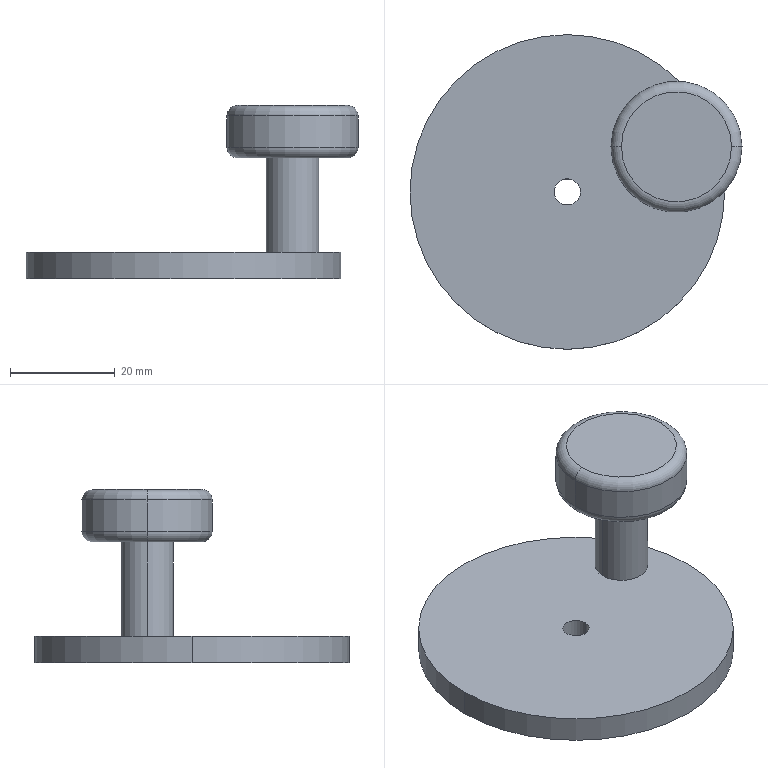Part | SolidWorks | features ICE 3, Extrusion 1, Fillet 1 | 1 solid | 16 faces | box 63.316 x 60 x 33 mm | volume 20231 mm3 | cylinder 8 | torus 4 | plane 4 | commonest cylinder face diameters 5 x2 10 x2 25 x2 60 x2
STEP:
#1=CARTESIAN_POINT('',(8.316,8.573,31.));
#2=VERTEX_POINT('',#1);
#3=CARTESIAN_POINT('',(33.316,8.573,31.));
#4=VERTEX_POINT('',#3);
#5=CARTESIAN_POINT('',(20.816,8.573,31.));
#6=DIRECTION('',(0.,0.,-1.));
#7=DIRECTION('',(1.,0.,0.));
#8=AXIS2_PLACEMENT_3D('',#5,#6,#7);
#9=CIRCLE('',#8,12.5);
#10=EDGE_CURVE('',#2,#4,#9,.T.);
#11=ORIENTED_EDGE('',*,*,#10,.F.);
#12=CARTESIAN_POINT('',(10.316,8.573,33.));
#13=VERTEX_POINT('',#12);
#14=CARTESIAN_POINT('',(10.316,8.573,31.));
#15=DIRECTION('',(0.,1.,0.));
#16=DIRECTION('',(-1.,0.,0.));
#17=AXIS2_PLACEMENT_3D('',#14,#15,#16);
#18=CIRCLE('',#17,2.);
#19=EDGE_CURVE('',#2,#13,#18,.T.);
#20=ORIENTED_EDGE('',*,*,#19,.T.);
#21=CARTESIAN_POINT('',(31.316,8.573,33.));
#22=VERTEX_POINT('',#21);
#23=CARTESIAN_POINT('',(20.816,8.573,33.));
#24=DIRECTION('',(0.,0.,1.));
#25=DIRECTION('',(1.,0.,0.));
#26=AXIS2_PLACEMENT_3D('',#23,#24,#25);
#27=CIRCLE('',#26,10.5);
#28=EDGE_CURVE('',#22,#13,#27,.T.);
#29=ORIENTED_EDGE('',*,*,#28,.F.);
#30=CARTESIAN_POINT('',(31.316,8.573,31.));
#31=DIRECTION('',(0.,-1.,0.));
#32=DIRECTION('',(0.,0.,-1.));
#33=AXIS2_PLACEMENT_3D('',#30,#31,#32);
#34=CIRCLE('',#33,2.);
#35=EDGE_CURVE('',#4,#22,#34,.T.);
#36=ORIENTED_EDGE('',*,*,#35,.F.);
#37=EDGE_LOOP('',(#11,#20,#29,#36));
#38=FACE_OUTER_BOUND('',#37,.T.);
#39=CARTESIAN_POINT('',(20.816,8.573,31.));
#40=DIRECTION('',(0.,0.,1.));
#41=DIRECTION('',(1.,0.,0.));
#42=AXIS2_PLACEMENT_3D('',#39,#40,#41);
#43=TOROIDAL_SURFACE('',#42,10.5,2.);
#44=ADVANCED_FACE('',(#38),#43,.T.);
#45=CARTESIAN_POINT('',(10.316,8.573,23.));
#46=VERTEX_POINT('',#45);
#47=CARTESIAN_POINT('',(31.316,8.573,23.));
#48=VERTEX_POINT('',#47);
#49=CARTESIAN_POINT('',(20.816,8.573,23.));
#50=DIRECTION('',(0.,0.,-1.));
#51=DIRECTION('',(1.,0.,0.));
#52=AXIS2_PLACEMENT_3D('',#49,#50,#51);
#53=CIRCLE('',#52,10.5);
#54=EDGE_CURVE('',#46,#48,#53,.T.);
#55=ORIENTED_EDGE('',*,*,#54,.F.);
#56=CARTESIAN_POINT('',(8.316,8.573,25.));
#57=VERTEX_POINT('',#56);
#58=CARTESIAN_POINT('',(10.316,8.573,25.));
#59=DIRECTION('',(0.,1.,0.));
#60=DIRECTION('',(-1.,0.,0.));
#61=AXIS2_PLACEMENT_3D('',#58,#59,#60);
#62=CIRCLE('',#61,2.);
#63=EDGE_CURVE('',#46,#57,#62,.T.);
#64=ORIENTED_EDGE('',*,*,#63,.T.);
#65=CARTESIAN_POINT('',(33.316,8.573,25.));
#66=VERTEX_POINT('',#65);
#67=CARTESIAN_POINT('',(20.816,8.573,25.));
#68=DIRECTION('',(0.,0.,1.));
#69=DIRECTION('',(1.,0.,0.));
#70=AXIS2_PLACEMENT_3D('',#67,#68,#69);
#71=CIRCLE('',#70,12.5);
#72=EDGE_CURVE('',#66,#57,#71,.T.);
#73=ORIENTED_EDGE('',*,*,#72,.F.);
#74=CARTESIAN_POINT('',(31.316,8.573,25.));
#75=DIRECTION('',(0.,-1.,0.));
#76=DIRECTION('',(0.,0.,-1.));
#77=AXIS2_PLACEMENT_3D('',#74,#75,#76);
#78=CIRCLE('',#77,2.);
#79=EDGE_CURVE('',#48,#66,#78,.T.);
#80=ORIENTED_EDGE('',*,*,#79,.F.);
#81=EDGE_LOOP('',(#55,#64,#73,#80));
#82=FACE_OUTER_BOUND('',#81,.T.);
#83=CARTESIAN_POINT('',(20.816,8.573,25.));
#84=DIRECTION('',(0.,0.,1.));
#85=DIRECTION('',(1.,0.,0.));
#86=AXIS2_PLACEMENT_3D('',#83,#84,#85);
#87=TOROIDAL_SURFACE('',#86,10.5,2.);
#88=ADVANCED_FACE('',(#82),#87,.T.);
#89=ORIENTED_EDGE('',*,*,#10,.T.);
#90=CARTESIAN_POINT('',(33.316,8.573,33.));
#91=DIRECTION('',(0.,0.,-1.));
#92=VECTOR('',#91,1000.);
#93=LINE('',#90,#92);
#94=EDGE_CURVE('',#4,#66,#93,.T.);
#95=ORIENTED_EDGE('',*,*,#94,.T.);
#96=ORIENTED_EDGE('',*,*,#72,.T.);
#97=CARTESIAN_POINT('',(8.316,8.573,33.));
#98=DIRECTION('',(0.,0.,-1.));
#99=VECTOR('',#98,1000.);
#100=LINE('',#97,#99);
#101=EDGE_CURVE('',#2,#57,#100,.T.);
#102=ORIENTED_EDGE('',*,*,#101,.F.);
#103=EDGE_LOOP('',(#89,#95,#96,#102));
#104=FACE_OUTER_BOUND('',#103,.T.);
#105=CARTESIAN_POINT('',(20.816,8.573,33.));
#106=DIRECTION('',(0.,0.,-1.));
#107=DIRECTION('',(-1.,0.,0.));
#108=AXIS2_PLACEMENT_3D('',#105,#106,#107);
#109=CYLINDRICAL_SURFACE('',#108,12.5);
#110=ADVANCED_FACE('',(#104),#109,.T.);
#111=CARTESIAN_POINT('',(25.816,8.573,23.));
#112=VERTEX_POINT('',#111);
#113=CARTESIAN_POINT('',(15.816,8.573,23.));
#114=VERTEX_POINT('',#113);
#115=CARTESIAN_POINT('',(20.816,8.573,23.));
#116=DIRECTION('',(0.,0.,1.));
#117=DIRECTION('',(1.,0.,0.));
#118=AXIS2_PLACEMENT_3D('',#115,#116,#117);
#119=CIRCLE('',#118,5.);
#120=EDGE_CURVE('',#112,#114,#119,.T.);
#121=ORIENTED_EDGE('',*,*,#120,.F.);
#122=CARTESIAN_POINT('',(25.816,8.573,5.));
#123=VERTEX_POINT('',#122);
#124=CARTESIAN_POINT('',(25.816,8.573,23.));
#125=DIRECTION('',(0.,0.,-1.));
#126=VECTOR('',#125,1000.);
#127=LINE('',#124,#126);
#128=EDGE_CURVE('',#112,#123,#127,.T.);
#129=ORIENTED_EDGE('',*,*,#128,.T.);
#130=CARTESIAN_POINT('',(15.816,8.573,5.));
#131=VERTEX_POINT('',#130);
#132=CARTESIAN_POINT('',(20.816,8.573,5.));
#133=DIRECTION('',(0.,0.,1.));
#134=DIRECTION('',(1.,0.,0.));
#135=AXIS2_PLACEMENT_3D('',#132,#133,#134);
#136=CIRCLE('',#135,5.);
#137=EDGE_CURVE('',#123,#131,#136,.T.);
#138=ORIENTED_EDGE('',*,*,#137,.T.);
#139=CARTESIAN_POINT('',(15.816,8.573,23.));
#140=DIRECTION('',(0.,0.,-1.));
#141=VECTOR('',#140,1000.);
#142=LINE('',#139,#141);
#143=EDGE_CURVE('',#114,#131,#142,.T.);
#144=ORIENTED_EDGE('',*,*,#143,.F.);
#145=EDGE_LOOP('',(#121,#129,#138,#144));
#146=FACE_OUTER_BOUND('',#145,.T.);
#147=CARTESIAN_POINT('',(20.816,8.573,23.));
#148=DIRECTION('',(0.,0.,-1.));
#149=DIRECTION('',(-1.,0.,0.));
#150=AXIS2_PLACEMENT_3D('',#147,#148,#149);
#151=CYLINDRICAL_SURFACE('',#150,5.);
#152=ADVANCED_FACE('',(#146),#151,.T.);
#153=CARTESIAN_POINT('',(-2.5,0.,0.));
#154=VERTEX_POINT('',#153);
#155=CARTESIAN_POINT('',(2.5,0.,0.));
#156=VERTEX_POINT('',#155);
#157=CARTESIAN_POINT('',(0.,0.,0.));
#158=DIRECTION('',(0.,0.,1.));
#159=DIRECTION('',(1.,0.,0.));
#160=AXIS2_PLACEMENT_3D('',#157,#158,#159);
#161=CIRCLE('',#160,2.5);
#162=EDGE_CURVE('',#154,#156,#161,.T.);
#163=ORIENTED_EDGE('',*,*,#162,.F.);
#164=CARTESIAN_POINT('',(-2.5,0.,5.));
#165=VERTEX_POINT('',#164);
#166=CARTESIAN_POINT('',(-2.5,0.,0.));
#167=DIRECTION('',(0.,0.,1.));
#168=VECTOR('',#167,1000.);
#169=LINE('',#166,#168);
#170=EDGE_CURVE('',#154,#165,#169,.T.);
#171=ORIENTED_EDGE('',*,*,#170,.T.);
#172=CARTESIAN_POINT('',(2.5,0.,5.));
#173=VERTEX_POINT('',#172);
#174=CARTESIAN_POINT('',(0.,0.,5.));
#175=DIRECTION('',(0.,0.,1.));
#176=DIRECTION('',(1.,0.,0.));
#177=AXIS2_PLACEMENT_3D('',#174,#175,#176);
#178=CIRCLE('',#177,2.5);
#179=EDGE_CURVE('',#165,#173,#178,.T.);
#180=ORIENTED_EDGE('',*,*,#179,.T.);
#181=CARTESIAN_POINT('',(2.5,0.,0.));
#182=DIRECTION('',(0.,0.,1.));
#183=VECTOR('',#182,1000.);
#184=LINE('',#181,#183);
#185=EDGE_CURVE('',#156,#173,#184,.T.);
#186=ORIENTED_EDGE('',*,*,#185,.F.);
#187=EDGE_LOOP('',(#163,#171,#180,#186));
#188=FACE_OUTER_BOUND('',#187,.T.);
#189=CARTESIAN_POINT('',(0.,0.,0.));
#190=DIRECTION('',(0.,0.,1.));
#191=DIRECTION('',(1.,0.,0.));
#192=AXIS2_PLACEMENT_3D('',#189,#190,#191);
#193=CYLINDRICAL_SURFACE('',#192,2.5);
#194=ADVANCED_FACE('',(#188),#193,.F.);
#195=CARTESIAN_POINT('',(30.,0.,5.));
#196=VERTEX_POINT('',#195);
#197=CARTESIAN_POINT('',(-30.,0.,5.));
#198=VERTEX_POINT('',#197);
#199=CARTESIAN_POINT('',(0.,0.,5.));
#200=DIRECTION('',(0.,0.,1.));
#201=DIRECTION('',(1.,0.,0.));
#202=AXIS2_PLACEMENT_3D('',#199,#200,#201);
#203=CIRCLE('',#202,30.);
#204=EDGE_CURVE('',#196,#198,#203,.T.);
#205=ORIENTED_EDGE('',*,*,#204,.F.);
#206=CARTESIAN_POINT('',(30.,0.,0.));
#207=VERTEX_POINT('',#206);
#208=CARTESIAN_POINT('',(30.,0.,5.));
#209=DIRECTION('',(0.,0.,-1.));
#210=VECTOR('',#209,1000.);
#211=LINE('',#208,#210);
#212=EDGE_CURVE('',#196,#207,#211,.T.);
#213=ORIENTED_EDGE('',*,*,#212,.T.);
#214=CARTESIAN_POINT('',(-30.,0.,0.));
#215=VERTEX_POINT('',#214);
#216=CARTESIAN_POINT('',(0.,0.,0.));
#217=DIRECTION('',(0.,0.,1.));
#218=DIRECTION('',(1.,0.,0.));
#219=AXIS2_PLACEMENT_3D('',#216,#217,#218);
#220=CIRCLE('',#219,30.);
#221=EDGE_CURVE('',#207,#215,#220,.T.);
#222=ORIENTED_EDGE('',*,*,#221,.T.);
#223=CARTESIAN_POINT('',(-30.,0.,5.));
#224=DIRECTION('',(0.,0.,-1.));
#225=VECTOR('',#224,1000.);
#226=LINE('',#223,#225);
#227=EDGE_CURVE('',#198,#215,#226,.T.);
#228=ORIENTED_EDGE('',*,*,#227,.F.);
#229=EDGE_LOOP('',(#205,#213,#222,#228));
#230=FACE_OUTER_BOUND('',#229,.T.);
#231=CARTESIAN_POINT('',(0.,0.,5.));
#232=DIRECTION('',(0.,0.,-1.));
#233=DIRECTION('',(-1.,0.,0.));
#234=AXIS2_PLACEMENT_3D('',#231,#232,#233);
#235=CYLINDRICAL_SURFACE('',#234,30.);
#236=ADVANCED_FACE('',(#230),#235,.T.);
#237=ORIENTED_EDGE('',*,*,#212,.F.);
#238=CARTESIAN_POINT('',(0.,0.,5.));
#239=DIRECTION('',(0.,0.,1.));
#240=DIRECTION('',(1.,0.,0.));
#241=AXIS2_PLACEMENT_3D('',#238,#239,#240);
#242=CIRCLE('',#241,30.);
#243=EDGE_CURVE('',#198,#196,#242,.T.);
#244=ORIENTED_EDGE('',*,*,#243,.F.);
#245=ORIENTED_EDGE('',*,*,#227,.T.);
#246=CARTESIAN_POINT('',(0.,0.,0.));
#247=DIRECTION('',(0.,0.,1.));
#248=DIRECTION('',(1.,0.,0.));
#249=AXIS2_PLACEMENT_3D('',#246,#247,#248);
#250=CIRCLE('',#249,30.);
#251=EDGE_CURVE('',#215,#207,#250,.T.);
#252=ORIENTED_EDGE('',*,*,#251,.T.);
#253=EDGE_LOOP('',(#237,#244,#245,#252));
#254=FACE_OUTER_BOUND('',#253,.T.);
#255=CARTESIAN_POINT('',(0.,0.,5.));
#256=DIRECTION('',(0.,0.,-1.));
#257=DIRECTION('',(-1.,0.,0.));
#258=AXIS2_PLACEMENT_3D('',#255,#256,#257);
#259=CYLINDRICAL_SURFACE('',#258,30.);
#260=ADVANCED_FACE('',(#254),#259,.T.);
#261=CARTESIAN_POINT('',(20.816,8.573,5.));
#262=DIRECTION('',(0.,0.,1.));
#263=DIRECTION('',(1.,0.,0.));
#264=AXIS2_PLACEMENT_3D('',#261,#262,#263);
#265=CIRCLE('',#264,5.);
#266=EDGE_CURVE('',#131,#123,#265,.T.);
#267=ORIENTED_EDGE('',*,*,#266,.F.);
#268=ORIENTED_EDGE('',*,*,#137,.F.);
#269=EDGE_LOOP('',(#267,#268));
#270=FACE_BOUND('',#269,.T.);
#271=CARTESIAN_POINT('',(0.,0.,5.));
#272=DIRECTION('',(0.,0.,1.));
#273=DIRECTION('',(1.,0.,0.));
#274=AXIS2_PLACEMENT_3D('',#271,#272,#273);
#275=CIRCLE('',#274,2.5);
#276=EDGE_CURVE('',#173,#165,#275,.T.);
#277=ORIENTED_EDGE('',*,*,#276,.F.);
#278=ORIENTED_EDGE('',*,*,#179,.F.);
#279=EDGE_LOOP('',(#277,#278));
#280=FACE_BOUND('',#279,.T.);
#281=ORIENTED_EDGE('',*,*,#243,.T.);
#282=ORIENTED_EDGE('',*,*,#204,.T.);
#283=EDGE_LOOP('',(#281,#282));
#284=FACE_OUTER_BOUND('',#283,.T.);
#285=CARTESIAN_POINT('',(0.,0.,5.));
#286=DIRECTION('',(0.,0.,1.));
#287=DIRECTION('',(1.,0.,0.));
#288=AXIS2_PLACEMENT_3D('',#285,#286,#287);
#289=PLANE('',#288);
#290=ADVANCED_FACE('',(#270,#280,#284),#289,.T.);
#291=CARTESIAN_POINT('',(0.,0.,0.));
#292=DIRECTION('',(0.,0.,1.));
#293=DIRECTION('',(1.,0.,0.));
#294=AXIS2_PLACEMENT_3D('',#291,#292,#293);
#295=CIRCLE('',#294,2.5);
#296=EDGE_CURVE('',#156,#154,#295,.T.);
#297=ORIENTED_EDGE('',*,*,#296,.T.);
#298=ORIENTED_EDGE('',*,*,#162,.T.);
#299=EDGE_LOOP('',(#297,#298));
#300=FACE_BOUND('',#299,.T.);
#301=ORIENTED_EDGE('',*,*,#251,.F.);
#302=ORIENTED_EDGE('',*,*,#221,.F.);
#303=EDGE_LOOP('',(#301,#302));
#304=FACE_OUTER_BOUND('',#303,.T.);
#305=CARTESIAN_POINT('',(0.,0.,0.));
#306=DIRECTION('',(0.,0.,1.));
#307=DIRECTION('',(1.,0.,0.));
#308=AXIS2_PLACEMENT_3D('',#305,#306,#307);
#309=PLANE('',#308);
#310=ADVANCED_FACE('',(#300,#304),#309,.F.);
#311=ORIENTED_EDGE('',*,*,#170,.F.);
#312=ORIENTED_EDGE('',*,*,#296,.F.);
#313=ORIENTED_EDGE('',*,*,#185,.T.);
#314=ORIENTED_EDGE('',*,*,#276,.T.);
#315=EDGE_LOOP('',(#311,#312,#313,#314));
#316=FACE_OUTER_BOUND('',#315,.T.);
#317=CARTESIAN_POINT('',(0.,0.,0.));
#318=DIRECTION('',(0.,0.,1.));
#319=DIRECTION('',(1.,0.,0.));
#320=AXIS2_PLACEMENT_3D('',#317,#318,#319);
#321=CYLINDRICAL_SURFACE('',#320,2.5);
#322=ADVANCED_FACE('',(#316),#321,.F.);
#323=ORIENTED_EDGE('',*,*,#128,.F.);
#324=CARTESIAN_POINT('',(20.816,8.573,23.));
#325=DIRECTION('',(0.,0.,1.));
#326=DIRECTION('',(1.,0.,0.));
#327=AXIS2_PLACEMENT_3D('',#324,#325,#326);
#328=CIRCLE('',#327,5.);
#329=EDGE_CURVE('',#114,#112,#328,.T.);
#330=ORIENTED_EDGE('',*,*,#329,.F.);
#331=ORIENTED_EDGE('',*,*,#143,.T.);
#332=ORIENTED_EDGE('',*,*,#266,.T.);
#333=EDGE_LOOP('',(#323,#330,#331,#332));
#334=FACE_OUTER_BOUND('',#333,.T.);
#335=CARTESIAN_POINT('',(20.816,8.573,23.));
#336=DIRECTION('',(0.,0.,-1.));
#337=DIRECTION('',(-1.,0.,0.));
#338=AXIS2_PLACEMENT_3D('',#335,#336,#337);
#339=CYLINDRICAL_SURFACE('',#338,5.);
#340=ADVANCED_FACE('',(#334),#339,.T.);
#341=ORIENTED_EDGE('',*,*,#94,.F.);
#342=CARTESIAN_POINT('',(20.816,8.573,31.));
#343=DIRECTION('',(0.,0.,-1.));
#344=DIRECTION('',(1.,0.,0.));
#345=AXIS2_PLACEMENT_3D('',#342,#343,#344);
#346=CIRCLE('',#345,12.5);
#347=EDGE_CURVE('',#4,#2,#346,.T.);
#348=ORIENTED_EDGE('',*,*,#347,.T.);
#349=ORIENTED_EDGE('',*,*,#101,.T.);
#350=CARTESIAN_POINT('',(20.816,8.573,25.));
#351=DIRECTION('',(0.,0.,1.));
#352=DIRECTION('',(1.,0.,0.));
#353=AXIS2_PLACEMENT_3D('',#350,#351,#352);
#354=CIRCLE('',#353,12.5);
#355=EDGE_CURVE('',#57,#66,#354,.T.);
#356=ORIENTED_EDGE('',*,*,#355,.T.);
#357=EDGE_LOOP('',(#341,#348,#349,#356));
#358=FACE_OUTER_BOUND('',#357,.T.);
#359=CARTESIAN_POINT('',(20.816,8.573,33.));
#360=DIRECTION('',(0.,0.,-1.));
#361=DIRECTION('',(-1.,0.,0.));
#362=AXIS2_PLACEMENT_3D('',#359,#360,#361);
#363=CYLINDRICAL_SURFACE('',#362,12.5);
#364=ADVANCED_FACE('',(#358),#363,.T.);
#365=ORIENTED_EDGE('',*,*,#28,.T.);
#366=CARTESIAN_POINT('',(20.816,8.573,33.));
#367=DIRECTION('',(0.,0.,1.));
#368=DIRECTION('',(1.,0.,0.));
#369=AXIS2_PLACEMENT_3D('',#366,#367,#368);
#370=CIRCLE('',#369,10.5);
#371=EDGE_CURVE('',#13,#22,#370,.T.);
#372=ORIENTED_EDGE('',*,*,#371,.T.);
#373=EDGE_LOOP('',(#365,#372));
#374=FACE_OUTER_BOUND('',#373,.T.);
#375=CARTESIAN_POINT('',(20.816,8.573,33.));
#376=DIRECTION('',(0.,0.,1.));
#377=DIRECTION('',(1.,0.,0.));
#378=AXIS2_PLACEMENT_3D('',#375,#376,#377);
#379=PLANE('',#378);
#380=ADVANCED_FACE('',(#374),#379,.T.);
#381=CARTESIAN_POINT('',(20.816,8.573,23.));
#382=DIRECTION('',(0.,0.,-1.));
#383=DIRECTION('',(1.,0.,0.));
#384=AXIS2_PLACEMENT_3D('',#381,#382,#383);
#385=CIRCLE('',#384,10.5);
#386=EDGE_CURVE('',#48,#46,#385,.T.);
#387=ORIENTED_EDGE('',*,*,#386,.T.);
#388=ORIENTED_EDGE('',*,*,#54,.T.);
#389=EDGE_LOOP('',(#387,#388));
#390=FACE_OUTER_BOUND('',#389,.T.);
#391=ORIENTED_EDGE('',*,*,#329,.T.);
#392=ORIENTED_EDGE('',*,*,#120,.T.);
#393=EDGE_LOOP('',(#391,#392));
#394=FACE_BOUND('',#393,.T.);
#395=CARTESIAN_POINT('',(20.816,8.573,23.));
#396=DIRECTION('',(0.,0.,1.));
#397=DIRECTION('',(1.,0.,0.));
#398=AXIS2_PLACEMENT_3D('',#395,#396,#397);
#399=PLANE('',#398);
#400=ADVANCED_FACE('',(#390,#394),#399,.F.);
#401=ORIENTED_EDGE('',*,*,#63,.F.);
#402=ORIENTED_EDGE('',*,*,#386,.F.);
#403=ORIENTED_EDGE('',*,*,#79,.T.);
#404=ORIENTED_EDGE('',*,*,#355,.F.);
#405=EDGE_LOOP('',(#401,#402,#403,#404));
#406=FACE_OUTER_BOUND('',#405,.T.);
#407=CARTESIAN_POINT('',(20.816,8.573,25.));
#408=DIRECTION('',(0.,0.,1.));
#409=DIRECTION('',(1.,0.,0.));
#410=AXIS2_PLACEMENT_3D('',#407,#408,#409);
#411=TOROIDAL_SURFACE('',#410,10.5,2.);
#412=ADVANCED_FACE('',(#406),#411,.T.);
#413=ORIENTED_EDGE('',*,*,#19,.F.);
#414=ORIENTED_EDGE('',*,*,#347,.F.);
#415=ORIENTED_EDGE('',*,*,#35,.T.);
#416=ORIENTED_EDGE('',*,*,#371,.F.);
#417=EDGE_LOOP('',(#413,#414,#415,#416));
#418=FACE_OUTER_BOUND('',#417,.T.);
#419=CARTESIAN_POINT('',(20.816,8.573,31.));
#420=DIRECTION('',(0.,0.,1.));
#421=DIRECTION('',(1.,0.,0.));
#422=AXIS2_PLACEMENT_3D('',#419,#420,#421);
#423=TOROIDAL_SURFACE('',#422,10.5,2.);
#424=ADVANCED_FACE('',(#418),#423,.T.);
#425=CLOSED_SHELL('',(#44,#88,#110,#152,#194,#236,#260,#290,#310,#322,#340,#364,#380,#400,#412,#424));
#426=MANIFOLD_SOLID_BREP('',#425);
#427=CARTESIAN_POINT('',(0.,0.,0.));
#428=DIRECTION('',(0.,0.,1.));
#429=DIRECTION('',(1.,0.,0.));
#430=AXIS2_PLACEMENT_3D('',#427,#428,#429);
#431=(LENGTH_UNIT()NAMED_UNIT(*)SI_UNIT(.MILLI.,.METRE.));
#432=UNCERTAINTY_MEASURE_WITH_UNIT(LENGTH_MEASURE(0.00001),#431,'','');
#433=(NAMED_UNIT(*)PLANE_ANGLE_UNIT()SI_UNIT($,.RADIAN.));
#434=(NAMED_UNIT(*)SI_UNIT($,.STERADIAN.)SOLID_ANGLE_UNIT());
#435=(GEOMETRIC_REPRESENTATION_CONTEXT(3)GLOBAL_UNCERTAINTY_ASSIGNED_CONTEXT((#432))GLOBAL_UNIT_ASSIGNED_CONTEXT((#431,#433,#434))REPRESENTATION_CONTEXT('',''));
#436=ADVANCED_BREP_SHAPE_REPRESENTATION('',(#426,#430),#435);